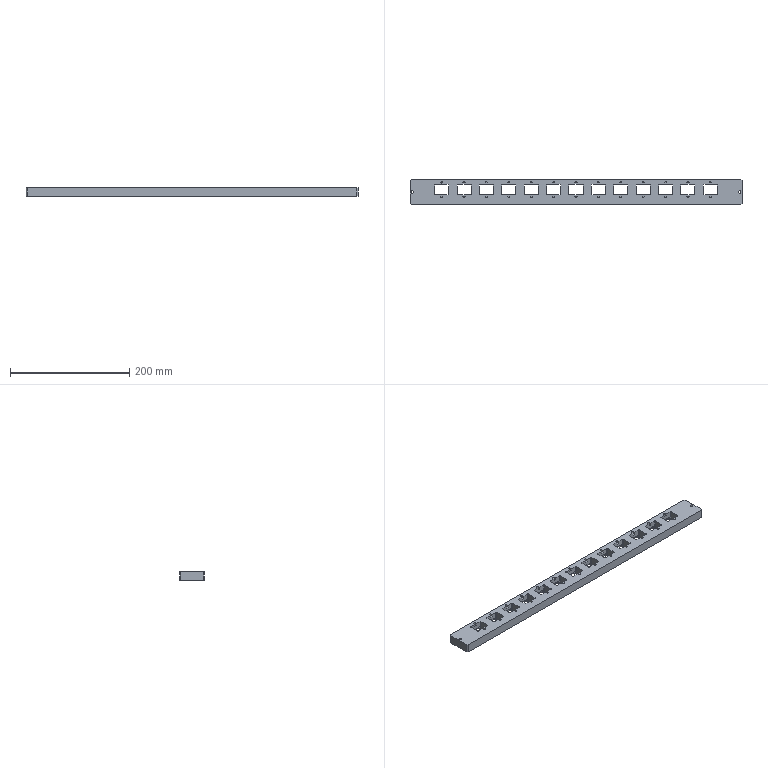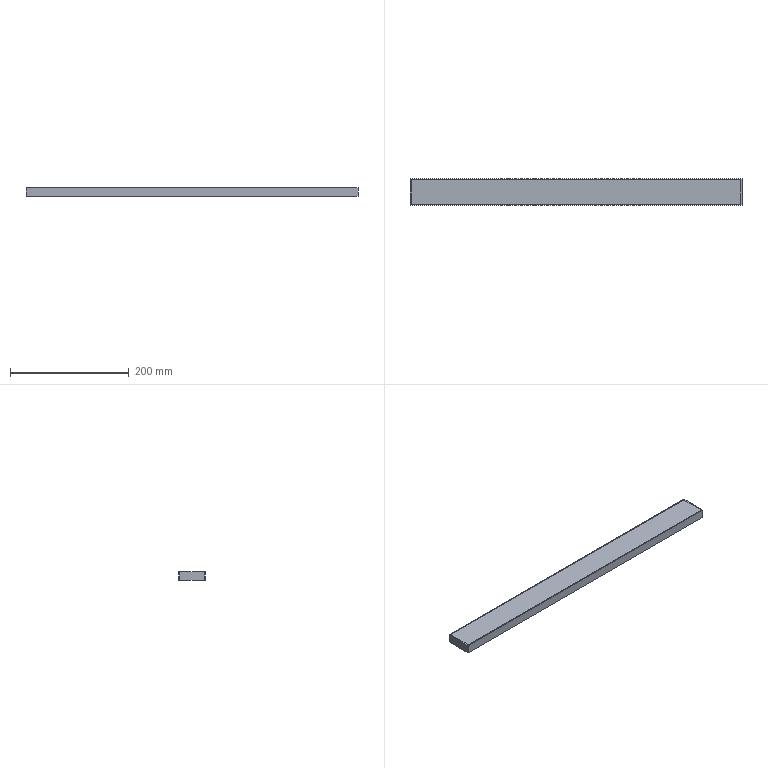CAM job | NX | 3-axis milling, drilling | part box 556 x 41 x 15 mm | stock box 560 x 45 x 15 mm
Tools:
number,name,description,diameter,corner_radius,flute_length,length,flutes
10,D10C,Milling Tool-5 Parameters,10.0,0.0,50.0,75.0,2
1,ZXZ,Milling Tool-5 Parameters,6.0,0.0,50.0,75.0,2
9,3.9ZT,Drilling Tool,3.9,0.0,35.0,50.0,2
8,4.0JD,Milling Tool-5 Parameters,4.0,0.0,30.0,30.0,4
3,D3,Milling Tool-5 Parameters,3.0,0.0,50.0,75.0,2
11,D10JING,Milling Tool-5 Parameters,10.0,0.0,50.0,75.0,2
6,D6JING,Milling Tool-5 Parameters,6.0,0.0,50.0,75.0,2
2,D2,Milling Tool-5 Parameters,2.0,0.0,50.0,75.0,2
12,D2JING,Milling Tool-5 Parameters,2.0,0.0,50.0,75.0,2
7,D6A45,Milling Tool-5 Parameters,6.0,0.0,50.0,75.0,2
Operations:
program,operation,operation_type,tool,method,geometry_group,spindle_rpm,surface_speed,feed_per_tooth,feed_cut,feed_plunge,cut_length_mm,path_length_mm,cut_time_min,machine_time_min
1,ZLEVEL_PROFILE,ZLevelMilling,D10C,METHOD,A,3500.0,109.0,0.3571,2500.0,1000.0,83099.313,83171.163,33.259,33.267
1,DRILLING,Operation,ZXZ,METHOD,A,3500.0,65.0,0.0357,250.0,0.0,8.0,627.008,0.032,0.0939
1,DRILLING_COPY,Operation,3.9ZT,METHOD,A,2000.0,24.0,0.0375,150.0,0.0,35.7,682.408,0.238,0.3027
1,HOLE_MILLING,CylinderMilling,D3,METHOD,A,5000.0,47.0,0.125,1250.0,100.0,162.569,886.269,0.1301,0.2024
1,DRILLING_COPY_COPY,Operation,4.0JD,METHOD,A,1000.0,12.0,0.0112,45.0,0.0,35.7,682.408,0.7933,0.858
1,ZLEVEL_PROFILE_COPY_1,ZLevelMilling,D10C,METHOD,A,3500.0,109.0,0.3571,2500.0,1000.0,37060.442,38450.316,15.08,15.219
1,ZLEVEL_PROFILE_COPY,ZLevelMilling,D10JING,METHOD,A,5000.0,157.0,0.1,1000.0,1000.0,1232.068,1315.768,1.232,1.24
1,ZLEVEL_PROFILE_COPY_1_COPY,ZLevelMilling,D6JING,METHOD,A,5000.0,94.0,0.18,1800.0,1000.0,30295.223,46001.146,19.721,21.292
1,ZLEVEL_PROFILE_COPY_1_COPY_COPY_1,ZLevelMilling,D6JING,METHOD,A,5000.0,94.0,0.11,1100.0,1000.0,807.735,4260.217,0.7367,1.082
1,ZLEVEL_PROFILE_COPY_1_COPY_COPY,ZLevelMilling,D2,METHOD,A,5000.0,47.0,0.12,1200.0,1000.0,14504.395,17999.814,12.236,12.585
1,ZLEVEL_PROFILE_COPY_1_COPY_COPY_2,ZLevelMilling,D2,METHOD,A,5000.0,31.0,0.11,1100.0,1000.0,71505.185,115430.742,65.656,70.049
1,PLANAR_MILL,PlanarMilling,D6A45,METHOD,A,7500.0,141.0,0.0933,1400.0,100.0,2489.753,3958.591,1.778,1.925
1,刀补,ZLevelMilling,D2JING,METHOD,A,5000.0,31.0,0.1,1000.0,1000.0,276.242,2660.409,0.2762,0.5147
2,ZLEVEL_PROFILE_COPY_1_COPY_COPY_3,ZLevelMilling,D6JING,METHOD,B,5000.0,94.0,0.18,1800.0,1000.0,13351.057,23082.778,8.164,9.137
2,ZLEVEL_PROFILE_COPY_1_COPY_COPY_2_COPY,ZLevelMilling,D2,METHOD,B,5000.0,31.0,0.11,1100.0,1000.0,34349.579,57525.714,31.542,33.86
2,PLANAR_MILL_COPY,PlanarMilling,D6A45,METHOD,B,7500.0,141.0,0.0933,1400.0,100.0,2437.753,3922.924,1.741,1.89
2,刀补_COPY,ZLevelMilling,D6JING,METHOD,B,5000.0,31.0,0.1,1000.0,1000.0,457.089,3314.274,0.4571,0.7428